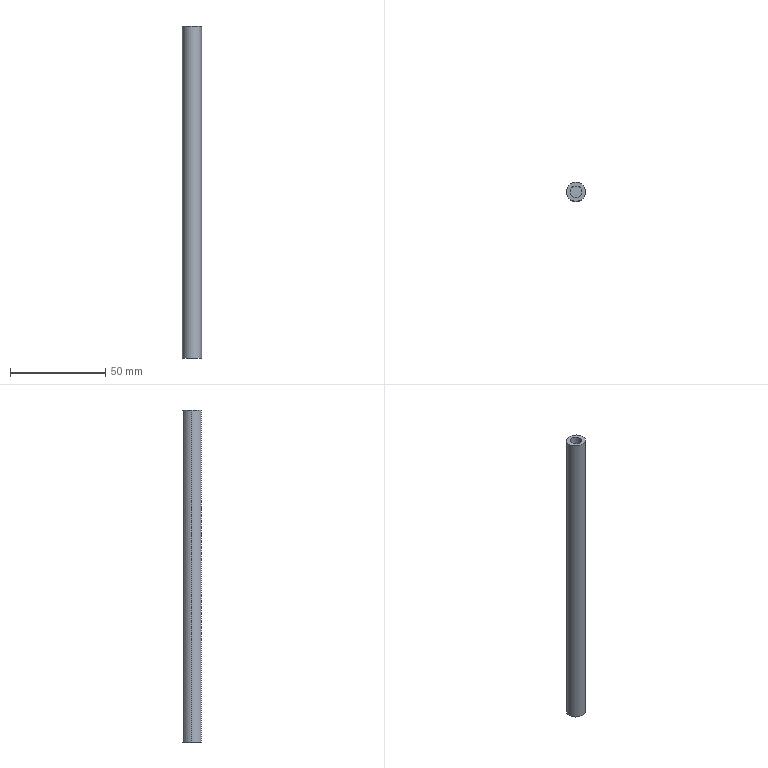Part | SolidWorks | features Extrusion 1, ICE 1, MirrorPattern 1 | 1 solid | 10 faces | box 10 x 10 x 174 mm | volume 13100 mm3 | cylinder 6 | plane 4 | commonest cylinder face diameters 6 x4 10 x2
STEP:
#1=CARTESIAN_POINT('',(-3.,0.,-77.));
#2=VERTEX_POINT('',#1);
#3=CARTESIAN_POINT('',(3.,0.,-77.));
#4=VERTEX_POINT('',#3);
#5=CARTESIAN_POINT('',(0.,0.,-77.));
#6=DIRECTION('',(0.,0.,1.));
#7=DIRECTION('',(1.,0.,0.));
#8=AXIS2_PLACEMENT_3D('',#5,#6,#7);
#9=CIRCLE('',#8,3.);
#10=EDGE_CURVE('',#2,#4,#9,.T.);
#11=ORIENTED_EDGE('',*,*,#10,.T.);
#12=CARTESIAN_POINT('',(3.,0.,-87.));
#13=VERTEX_POINT('',#12);
#14=CARTESIAN_POINT('',(3.,0.,-77.));
#15=DIRECTION('',(0.,0.,-1.));
#16=VECTOR('',#15,1000.);
#17=LINE('',#14,#16);
#18=EDGE_CURVE('',#4,#13,#17,.T.);
#19=ORIENTED_EDGE('',*,*,#18,.T.);
#20=CARTESIAN_POINT('',(-3.,0.,-87.));
#21=VERTEX_POINT('',#20);
#22=CARTESIAN_POINT('',(0.,0.,-87.));
#23=DIRECTION('',(0.,0.,1.));
#24=DIRECTION('',(1.,0.,0.));
#25=AXIS2_PLACEMENT_3D('',#22,#23,#24);
#26=CIRCLE('',#25,3.);
#27=EDGE_CURVE('',#21,#13,#26,.T.);
#28=ORIENTED_EDGE('',*,*,#27,.F.);
#29=CARTESIAN_POINT('',(-3.,0.,-77.));
#30=DIRECTION('',(0.,0.,-1.));
#31=VECTOR('',#30,1000.);
#32=LINE('',#29,#31);
#33=EDGE_CURVE('',#2,#21,#32,.T.);
#34=ORIENTED_EDGE('',*,*,#33,.F.);
#35=EDGE_LOOP('',(#11,#19,#28,#34));
#36=FACE_OUTER_BOUND('',#35,.T.);
#37=CARTESIAN_POINT('',(0.,0.,-77.));
#38=DIRECTION('',(0.,0.,-1.));
#39=DIRECTION('',(-1.,0.,0.));
#40=AXIS2_PLACEMENT_3D('',#37,#38,#39);
#41=CYLINDRICAL_SURFACE('',#40,3.);
#42=ADVANCED_FACE('',(#36),#41,.F.);
#43=CARTESIAN_POINT('',(-3.,0.,77.));
#44=VERTEX_POINT('',#43);
#45=CARTESIAN_POINT('',(3.,0.,77.));
#46=VERTEX_POINT('',#45);
#47=CARTESIAN_POINT('',(0.,0.,77.));
#48=DIRECTION('',(0.,0.,1.));
#49=DIRECTION('',(1.,0.,0.));
#50=AXIS2_PLACEMENT_3D('',#47,#48,#49);
#51=CIRCLE('',#50,3.);
#52=EDGE_CURVE('',#44,#46,#51,.T.);
#53=ORIENTED_EDGE('',*,*,#52,.F.);
#54=CARTESIAN_POINT('',(-3.,0.,87.));
#55=VERTEX_POINT('',#54);
#56=CARTESIAN_POINT('',(-3.,0.,77.));
#57=DIRECTION('',(0.,0.,1.));
#58=VECTOR('',#57,1000.);
#59=LINE('',#56,#58);
#60=EDGE_CURVE('',#44,#55,#59,.T.);
#61=ORIENTED_EDGE('',*,*,#60,.T.);
#62=CARTESIAN_POINT('',(3.,0.,87.));
#63=VERTEX_POINT('',#62);
#64=CARTESIAN_POINT('',(0.,0.,87.));
#65=DIRECTION('',(0.,0.,1.));
#66=DIRECTION('',(1.,0.,0.));
#67=AXIS2_PLACEMENT_3D('',#64,#65,#66);
#68=CIRCLE('',#67,3.);
#69=EDGE_CURVE('',#55,#63,#68,.T.);
#70=ORIENTED_EDGE('',*,*,#69,.T.);
#71=CARTESIAN_POINT('',(3.,0.,77.));
#72=DIRECTION('',(0.,0.,1.));
#73=VECTOR('',#72,1000.);
#74=LINE('',#71,#73);
#75=EDGE_CURVE('',#46,#63,#74,.T.);
#76=ORIENTED_EDGE('',*,*,#75,.F.);
#77=EDGE_LOOP('',(#53,#61,#70,#76));
#78=FACE_OUTER_BOUND('',#77,.T.);
#79=CARTESIAN_POINT('',(0.,0.,77.));
#80=DIRECTION('',(0.,0.,1.));
#81=DIRECTION('',(1.,0.,0.));
#82=AXIS2_PLACEMENT_3D('',#79,#80,#81);
#83=CYLINDRICAL_SURFACE('',#82,3.);
#84=ADVANCED_FACE('',(#78),#83,.F.);
#85=CARTESIAN_POINT('',(5.,0.,87.));
#86=VERTEX_POINT('',#85);
#87=CARTESIAN_POINT('',(-5.,0.,87.));
#88=VERTEX_POINT('',#87);
#89=CARTESIAN_POINT('',(0.,0.,87.));
#90=DIRECTION('',(0.,0.,1.));
#91=DIRECTION('',(1.,0.,0.));
#92=AXIS2_PLACEMENT_3D('',#89,#90,#91);
#93=CIRCLE('',#92,5.);
#94=EDGE_CURVE('',#86,#88,#93,.T.);
#95=ORIENTED_EDGE('',*,*,#94,.F.);
#96=CARTESIAN_POINT('',(5.,0.,-87.));
#97=VERTEX_POINT('',#96);
#98=CARTESIAN_POINT('',(5.,0.,87.));
#99=DIRECTION('',(0.,0.,-1.));
#100=VECTOR('',#99,1000.);
#101=LINE('',#98,#100);
#102=EDGE_CURVE('',#86,#97,#101,.T.);
#103=ORIENTED_EDGE('',*,*,#102,.T.);
#104=CARTESIAN_POINT('',(-5.,0.,-87.));
#105=VERTEX_POINT('',#104);
#106=CARTESIAN_POINT('',(0.,0.,-87.));
#107=DIRECTION('',(0.,0.,1.));
#108=DIRECTION('',(1.,0.,0.));
#109=AXIS2_PLACEMENT_3D('',#106,#107,#108);
#110=CIRCLE('',#109,5.);
#111=EDGE_CURVE('',#97,#105,#110,.T.);
#112=ORIENTED_EDGE('',*,*,#111,.T.);
#113=CARTESIAN_POINT('',(-5.,0.,87.));
#114=DIRECTION('',(0.,0.,-1.));
#115=VECTOR('',#114,1000.);
#116=LINE('',#113,#115);
#117=EDGE_CURVE('',#88,#105,#116,.T.);
#118=ORIENTED_EDGE('',*,*,#117,.F.);
#119=EDGE_LOOP('',(#95,#103,#112,#118));
#120=FACE_OUTER_BOUND('',#119,.T.);
#121=CARTESIAN_POINT('',(0.,0.,87.));
#122=DIRECTION('',(0.,0.,-1.));
#123=DIRECTION('',(-1.,0.,0.));
#124=AXIS2_PLACEMENT_3D('',#121,#122,#123);
#125=CYLINDRICAL_SURFACE('',#124,5.);
#126=ADVANCED_FACE('',(#120),#125,.T.);
#127=CARTESIAN_POINT('',(0.,0.,-87.));
#128=DIRECTION('',(0.,0.,1.));
#129=DIRECTION('',(1.,0.,0.));
#130=AXIS2_PLACEMENT_3D('',#127,#128,#129);
#131=CIRCLE('',#130,5.);
#132=EDGE_CURVE('',#105,#97,#131,.T.);
#133=ORIENTED_EDGE('',*,*,#132,.F.);
#134=ORIENTED_EDGE('',*,*,#111,.F.);
#135=EDGE_LOOP('',(#133,#134));
#136=FACE_OUTER_BOUND('',#135,.T.);
#137=ORIENTED_EDGE('',*,*,#27,.T.);
#138=CARTESIAN_POINT('',(0.,0.,-87.));
#139=DIRECTION('',(0.,0.,1.));
#140=DIRECTION('',(1.,0.,0.));
#141=AXIS2_PLACEMENT_3D('',#138,#139,#140);
#142=CIRCLE('',#141,3.);
#143=EDGE_CURVE('',#13,#21,#142,.T.);
#144=ORIENTED_EDGE('',*,*,#143,.T.);
#145=EDGE_LOOP('',(#137,#144));
#146=FACE_BOUND('',#145,.T.);
#147=CARTESIAN_POINT('',(0.,0.,-87.));
#148=DIRECTION('',(0.,0.,1.));
#149=DIRECTION('',(1.,0.,0.));
#150=AXIS2_PLACEMENT_3D('',#147,#148,#149);
#151=PLANE('',#150);
#152=ADVANCED_FACE('',(#136,#146),#151,.F.);
#153=ORIENTED_EDGE('',*,*,#102,.F.);
#154=CARTESIAN_POINT('',(0.,0.,87.));
#155=DIRECTION('',(0.,0.,1.));
#156=DIRECTION('',(1.,0.,0.));
#157=AXIS2_PLACEMENT_3D('',#154,#155,#156);
#158=CIRCLE('',#157,5.);
#159=EDGE_CURVE('',#88,#86,#158,.T.);
#160=ORIENTED_EDGE('',*,*,#159,.F.);
#161=ORIENTED_EDGE('',*,*,#117,.T.);
#162=ORIENTED_EDGE('',*,*,#132,.T.);
#163=EDGE_LOOP('',(#153,#160,#161,#162));
#164=FACE_OUTER_BOUND('',#163,.T.);
#165=CARTESIAN_POINT('',(0.,0.,87.));
#166=DIRECTION('',(0.,0.,-1.));
#167=DIRECTION('',(-1.,0.,0.));
#168=AXIS2_PLACEMENT_3D('',#165,#166,#167);
#169=CYLINDRICAL_SURFACE('',#168,5.);
#170=ADVANCED_FACE('',(#164),#169,.T.);
#171=CARTESIAN_POINT('',(0.,0.,87.));
#172=DIRECTION('',(0.,0.,1.));
#173=DIRECTION('',(1.,0.,0.));
#174=AXIS2_PLACEMENT_3D('',#171,#172,#173);
#175=CIRCLE('',#174,3.);
#176=EDGE_CURVE('',#63,#55,#175,.T.);
#177=ORIENTED_EDGE('',*,*,#176,.F.);
#178=ORIENTED_EDGE('',*,*,#69,.F.);
#179=EDGE_LOOP('',(#177,#178));
#180=FACE_BOUND('',#179,.T.);
#181=ORIENTED_EDGE('',*,*,#159,.T.);
#182=ORIENTED_EDGE('',*,*,#94,.T.);
#183=EDGE_LOOP('',(#181,#182));
#184=FACE_OUTER_BOUND('',#183,.T.);
#185=CARTESIAN_POINT('',(0.,0.,87.));
#186=DIRECTION('',(0.,0.,1.));
#187=DIRECTION('',(1.,0.,0.));
#188=AXIS2_PLACEMENT_3D('',#185,#186,#187);
#189=PLANE('',#188);
#190=ADVANCED_FACE('',(#180,#184),#189,.T.);
#191=ORIENTED_EDGE('',*,*,#60,.F.);
#192=CARTESIAN_POINT('',(0.,0.,77.));
#193=DIRECTION('',(0.,0.,1.));
#194=DIRECTION('',(1.,0.,0.));
#195=AXIS2_PLACEMENT_3D('',#192,#193,#194);
#196=CIRCLE('',#195,3.);
#197=EDGE_CURVE('',#46,#44,#196,.T.);
#198=ORIENTED_EDGE('',*,*,#197,.F.);
#199=ORIENTED_EDGE('',*,*,#75,.T.);
#200=ORIENTED_EDGE('',*,*,#176,.T.);
#201=EDGE_LOOP('',(#191,#198,#199,#200));
#202=FACE_OUTER_BOUND('',#201,.T.);
#203=CARTESIAN_POINT('',(0.,0.,77.));
#204=DIRECTION('',(0.,0.,1.));
#205=DIRECTION('',(1.,0.,0.));
#206=AXIS2_PLACEMENT_3D('',#203,#204,#205);
#207=CYLINDRICAL_SURFACE('',#206,3.);
#208=ADVANCED_FACE('',(#202),#207,.F.);
#209=ORIENTED_EDGE('',*,*,#197,.T.);
#210=ORIENTED_EDGE('',*,*,#52,.T.);
#211=EDGE_LOOP('',(#209,#210));
#212=FACE_OUTER_BOUND('',#211,.T.);
#213=CARTESIAN_POINT('',(0.,0.,77.));
#214=DIRECTION('',(0.,0.,1.));
#215=DIRECTION('',(1.,0.,0.));
#216=AXIS2_PLACEMENT_3D('',#213,#214,#215);
#217=PLANE('',#216);
#218=ADVANCED_FACE('',(#212),#217,.T.);
#219=ORIENTED_EDGE('',*,*,#18,.F.);
#220=CARTESIAN_POINT('',(0.,0.,-77.));
#221=DIRECTION('',(0.,0.,1.));
#222=DIRECTION('',(1.,0.,0.));
#223=AXIS2_PLACEMENT_3D('',#220,#221,#222);
#224=CIRCLE('',#223,3.);
#225=EDGE_CURVE('',#4,#2,#224,.T.);
#226=ORIENTED_EDGE('',*,*,#225,.T.);
#227=ORIENTED_EDGE('',*,*,#33,.T.);
#228=ORIENTED_EDGE('',*,*,#143,.F.);
#229=EDGE_LOOP('',(#219,#226,#227,#228));
#230=FACE_OUTER_BOUND('',#229,.T.);
#231=CARTESIAN_POINT('',(0.,0.,-77.));
#232=DIRECTION('',(0.,0.,-1.));
#233=DIRECTION('',(-1.,0.,0.));
#234=AXIS2_PLACEMENT_3D('',#231,#232,#233);
#235=CYLINDRICAL_SURFACE('',#234,3.);
#236=ADVANCED_FACE('',(#230),#235,.F.);
#237=ORIENTED_EDGE('',*,*,#10,.F.);
#238=ORIENTED_EDGE('',*,*,#225,.F.);
#239=EDGE_LOOP('',(#237,#238));
#240=FACE_OUTER_BOUND('',#239,.T.);
#241=CARTESIAN_POINT('',(0.,0.,-77.));
#242=DIRECTION('',(0.,0.,-1.));
#243=DIRECTION('',(1.,0.,0.));
#244=AXIS2_PLACEMENT_3D('',#241,#242,#243);
#245=PLANE('',#244);
#246=ADVANCED_FACE('',(#240),#245,.T.);
#247=CLOSED_SHELL('',(#42,#84,#126,#152,#170,#190,#208,#218,#236,#246));
#248=MANIFOLD_SOLID_BREP('',#247);
#249=CARTESIAN_POINT('',(0.,0.,0.));
#250=DIRECTION('',(0.,0.,1.));
#251=DIRECTION('',(1.,0.,0.));
#252=AXIS2_PLACEMENT_3D('',#249,#250,#251);
#253=(LENGTH_UNIT()NAMED_UNIT(*)SI_UNIT(.MILLI.,.METRE.));
#254=UNCERTAINTY_MEASURE_WITH_UNIT(LENGTH_MEASURE(0.00001),#253,'','');
#255=(NAMED_UNIT(*)PLANE_ANGLE_UNIT()SI_UNIT($,.RADIAN.));
#256=(NAMED_UNIT(*)SI_UNIT($,.STERADIAN.)SOLID_ANGLE_UNIT());
#257=(GEOMETRIC_REPRESENTATION_CONTEXT(3)GLOBAL_UNCERTAINTY_ASSIGNED_CONTEXT((#254))GLOBAL_UNIT_ASSIGNED_CONTEXT((#253,#255,#256))REPRESENTATION_CONTEXT('',''));
#258=ADVANCED_BREP_SHAPE_REPRESENTATION('',(#248,#252),#257);